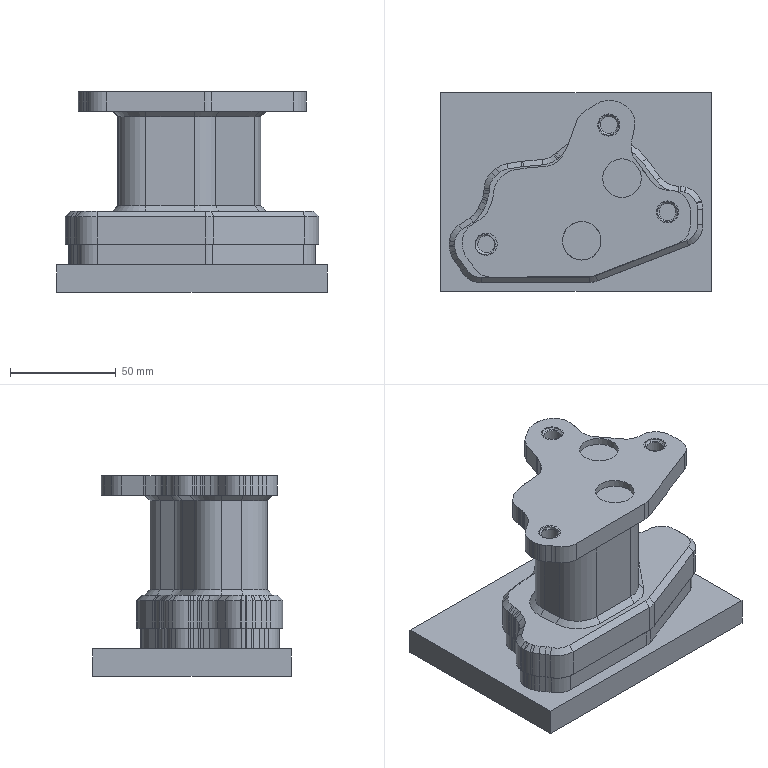NC program | NX | posted by the shop | part box 128.162 x 94.109 x 95 mm
Lines 31063 to 32055 of 131503:
31062 TOOL CALL 10 Z S8000
31063 CALL LBL101
31064 M3 M8
31065 M51
31066 CYCL DEF 32.0 TOLERANCE
31067 CYCL DEF 32.1 T0.012
31068 CYCL DEF 32.2 HSC-MODE:0
31069 L M126
31070 PLANE SPATIAL SPA-90. SPB+0.0 SPC-179.758 TURN FMAX SEQ-
31071 L X28.6141 Y32.9464 FMAX
31072 L Z140. FMAX
31073 L X28.614 Z35.4807 FMAX
31074 L X25.014 F1000.
31075 L Y14.5684
31076 L X24.4525 Y14.6761
31077 L X23.2391 Y14.816
31078 L X22.072 Y14.8611
31079 L X22.014
31080 L X-1.056
31081 L X-1.973 Y14.8323
31082 L X-2.9301 Y14.7461
31083 L X-3.8765 Y14.6024
31084 L X-4.0089 Y14.5747
31085 L Y51.3242
31086 L X-3.4472 Y51.2166
31087 L X-2.234 Y51.0768
31088 L X-1.0669 Y51.0316
31089 L X-1.0089
31090 L X22.0611
31091 L X22.9781 Y51.0604
31092 L X23.9352 Y51.1467
31093 L X24.8816 Y51.2903
31094 L X25.014 Y51.318
31095 L Y32.9464
31096 L X22.014
31097 L Y17.8611
31098 L X-1.0089
31099 L Y48.0316
31100 L X22.014
31101 L Y32.9464
31102 L X19.014
31103 L Y20.8611
31104 L X1.9911
31105 L Y45.0316
31106 L X19.014
31107 L Y32.9464
31108 L X16.014
31109 L Y23.8611
31110 L X4.9911
31111 L Y42.0316
31112 L X16.014
31113 L Y32.9464
31114 L X13.014
31115 L Y26.8611
31116 L X7.9911
31117 L Y39.0316
31118 L X10.4911
31119 L Y36.5316
31120 L X10.514
31121 L Y29.3611
31122 L X10.4911
31123 L Y36.5316
31124 L Y39.0316
31125 L X13.014
31126 L Y32.9464
31127 L X16.614
31128 L Z140. FMAX
31129 PLANE RESET STAY
31130 * - OPERATION: 新底壁铣_1_COPY - TOOL: T10 J-D6R0.5
31131 CALL LBL101
31132 CYCL DEF 32.0 TOLERANCE
31133 CYCL DEF 32.1 T0.012
31134 CYCL DEF 32.2 HSC-MODE:0
31135 PLANE SPATIAL SPA-90. SPB+0.0 SPC-3.662 TURN FMAX SEQ-
31136 L X1.7819 Y32.9464 FMAX
31137 L Z140. FMAX
31138 L X1.7818 Z20.4544 FMAX
31139 L X5.3818 F1000.
31140 L Y51.3246
31141 L X5.9427 Y51.2171
31142 L X7.1562 Y51.0765
31143 L X8.3242 Y51.0316
31144 L X8.3818
31145 L X14.9774
31146 L X15.8945 Y51.0604
31147 L X16.8516 Y51.1467
31148 L X17.798 Y51.2903
31149 L X17.9304 Y51.318
31150 L Y14.5685
31151 L X17.3687 Y14.6761
31152 L X16.1555 Y14.816
31153 L X14.9884 Y14.8611
31154 L X14.9304
31155 L X8.3347
31156 L X7.4177 Y14.8323
31157 L X6.4606 Y14.7461
31158 L X5.5141 Y14.6024
31159 L X5.3818 Y14.5747
31160 L Y32.9464
31161 L X8.3818
31162 L Y48.0316
31163 L X14.9304
31164 L Y17.8611
31165 L X8.3818
31166 L Y32.9464
31167 L X11.3818
31168 L Y45.0316
31169 L X11.9304
31170 L Y20.8611
31171 L X11.3818
31172 L Y32.9464
31173 L X7.7818
31174 L Z140. FMAX
31175 PLANE RESET STAY
31176 * - OPERATION: 等高混合 - TOOL: T10 J-D6R0.5
31177 CALL LBL101
31178 CYCL DEF 32.0 TOLERANCE
31179 CYCL DEF 32.1 T0.006
31180 CYCL DEF 32.2 HSC-MODE:0
31181 PLANE SPATIAL SPA-90. SPB+0.0 SPC+0.0 TURN FMAX SEQ-
31182 L X13.296 Y14.3074 FMAX
31183 L Z83.7547 FMAX
31184 L Z43.2547 FMAX
31185 CC X15.296 Y14.3211
31186 C X15.296 Y12.3211 DR+ F250.
31187 L X16.7642 F2500.
31188 L X16.8776 Y12.3206 Z43.247
31189 L X16.9909 Y12.3211 Z43.2393
31190 L X17.1042 Z43.2316
31191 L X17.2176 Z43.2239
31192 L X17.3309 Y12.3204 Z43.2162
31193 L X17.4442 Y12.3211 Z43.2085
31194 L X17.5576 Z43.2008
31195 L X17.6709 Z43.1932
31196 L X17.7842 Y12.3205 Z43.1855
31197 L X17.8976 Y12.3211 Z43.1778
31198 L X18.0109 Z43.1701
31199 L X18.1242 Z43.1624
31200 L X18.2375 Z43.1547
31201 L X13.5829
31202 L X13.5432 Y12.3207
31203 L X13.4221 Y12.3211 Z43.1347
31204 L X13.0586 Z43.0747
31205 L X12.9374 Y12.3206 Z43.0547
31206 L X13.0935 Y12.3211
31207 L X18.7348
31208 L X18.8509 Y12.3205
31209 L X18.9714 Y12.3211 Z43.0297
31210 L X19.0919 Z43.0047
31211 L X19.2123 Z42.9797
31212 L X19.3328 Y12.3205 Z42.9547
31213 L X12.4526 Y12.3204
31214 L X12.3573 Y12.3211 Z42.9297
31215 L X12.262 Z42.9047
31216 L X12.1667 Z42.8797
31217 L X12.0714 Z42.8547
31218 L X19.7213 Y12.3207
31219 L X19.8299 Y12.3204 Z42.8214
31220 L X19.9385 Y12.3211 Z42.788
31221 L X20.0471 Y12.3201 Z42.7547
31222 L X11.7317 Y12.3199
31223 L X11.6327 Y12.3211 Z42.7214
31224 L X11.5338 Z42.688
31225 L X11.4348 Y12.3203 Z42.6547
31226 L X20.3518 Y12.3201
31227 L X20.4405 Y12.321 Z42.6214
31228 L X20.5292 Z42.588
31229 L X20.6179 Y12.3202 Z42.5547
31230 L X20.4789 Y12.3211
31231 L X16.8018
31232 L X15.1344
31233 L X11.1511 Y12.321
31234 L X11.0302 Z42.5047
31235 L X10.9092 Z42.4547
31236 L X13.5853 Y12.3211
31237 L X18.2187
31238 L X20.7078
31239 L X20.859 Y12.3198
31240 L X20.941 Y12.3211 Z42.4214
31241 L X21.023 Z42.388
31242 L X21.1049 Z42.3547
31243 L X18.8143
31244 L X12.9705
31245 L X10.9568
31246 L X10.6732 Y12.3207
31247 L X10.5642 Y12.3209 Z42.3047
31248 L X10.4553 Y12.3201 Z42.2547
31249 L X10.6464 Y12.3211
31250 L X12.5219
31251 L X19.2578
31252 L X21.1691
31253 L X21.3186 Y12.3207
31254 L X21.4254 Y12.321 Z42.2047
31255 L X21.5322 Y12.3211 Z42.1547
31256 L X19.624
31257 L X12.1519
31258 L X10.4016
31259 L X10.2511 Y12.3194
31260 L X10.1521 Y12.321 Z42.1047
31261 L X10.0532 Y12.3193 Z42.0547
31262 L X10.1569 Y12.3211
31263 L X11.8326
31264 L X19.9416
31265 L X21.7212
31266 L X21.8126 Y12.3209 Z42.0047
31267 L X21.9041 Y12.3211 Z41.9547
31268 L X20.226
31269 L X11.5476
31270 L X9.9122
31271 L X9.864 Y12.3206
31272 L X9.7776 Y12.321 Z41.9047
31273 L X9.6912 Y12.3206 Z41.8547
31274 L X9.8348 Y12.3211
31275 L X11.2888
31276 L X20.4836
31277 L X22.0868 Y12.3209
31278 L X22.1732 Z41.8047
31279 L X22.2597 Z41.7547
31280 L X20.7218 Y12.3211
31281 L X11.0504
31282 L X9.6675
31283 L X9.5185 Y12.3193
31284 L X9.4347 Y12.321 Z41.7047
31285 L X9.351 Y12.3194 Z41.6547
31286 L X9.4228 Y12.3211
31287 L X10.8296
31288 L X20.9423
31289 L X22.413
31290 L X22.4297 Y12.3206
31291 L X22.5147 Y12.3209 Z41.6047
31292 L X22.5998 Y12.3207 Z41.5547
31293 L X22.5756 Y12.3211
31294 L X21.1501
31295 L X10.6218
31296 L X9.1898 Y12.3209
31297 L X9.1092 Y12.3204 Z41.5047
31298 L X9.0287 Y12.3192 Z41.4547
31299 L X9.1781 Y12.3211
31300 L X10.4257
31301 L X21.3451
31302 L X22.7571
31303 L X22.7724 Y12.3206
31304 L X22.8646 Y12.3204 Z41.4047
31305 L X22.9567 Y12.3196 Z41.3547
31306 L X22.8821 Y12.3211
31307 L X21.53
31308 L X10.2409
31309 L X8.9334
31310 L X8.8676 Y12.3195
31311 L X8.787 Y12.321 Z41.3047
31312 L X8.7064 Y12.3207 Z41.2547
31313 L X9.9122 Y12.3211
31314 L X10.0649
31315 L X21.7063
31316 L X23.0792 Y12.3209
31317 L X23.1794 Y12.3211 Z41.2047
31318 L X23.2797 Z41.1547
31319 L X21.8772
31320 L X9.8967
31321 L X8.6886
31322 L X8.5453 Y12.3192
31323 L X8.4647 Y12.321 Z41.1047
31324 L X8.3842 Y12.3196 Z41.0547
31325 L X8.4439 Y12.3211
31326 L X9.734
31327 L X22.0472
31328 L X23.4515 Y12.321
31329 L X23.5331 Y12.3209 Z41.0047
31330 L X23.6147 Y12.3207 Z40.9547
31331 L X22.2172 Y12.3211
31332 L X9.5728
31333 L X8.4439
31334 L X8.223 Y12.3206
31335 L X8.1425 Y12.3204 Z40.9047
31336 L X8.0619 Y12.3191 Z40.8547
31337 L X8.1992 Y12.3211
31338 L X9.4117
31339 L X22.3872
31340 L X23.7652
31341 L X23.8439 Y12.321 Z40.8047
31342 L X23.9227 Y12.3211 Z40.7547
31343 L X22.5572
31344 L X9.2506
31345 L X7.9008
31346 L X7.8202 Y12.3203 Z40.7047
31347 L X7.7397 Y12.3204 Z40.6547
31348 L X7.8982 Y12.3211
31349 L X9.0895
31350 L X22.7272
31351 L X24.0581
31352 L X24.1287 Y12.321 Z40.6047
31353 L X24.1994 Y12.3211 Z40.5547
31354 L X22.8972
31355 L X8.9283
31356 L X7.7098
31357 L X7.5786 Y12.3191
31358 L X7.498 Y12.321 Z40.5047
31359 L X7.4174 Y12.3198 Z40.4547
31360 L X7.4651 Y12.3211
31361 L X8.7672
31362 L X23.0659
31363 L X24.3368 Y12.321
31364 L X24.4048 Z40.4047
31365 L X24.4729 Y12.3211 Z40.3547
31366 L X23.2294
31367 L X8.6061
31368 L X7.4651
31369 L X7.2563 Y12.3202
31370 L X7.1686 Y12.3209 Z40.3047
31371 L X7.0809 Y12.3187 Z40.2547
31372 L X7.2203 Y12.3211
31373 L X8.445
31374 L X23.3859
31375 L X24.5946
31376 L X24.715 Y12.3208 Z40.1547
31377 L X23.5361 Y12.3211
31378 L X8.2838
31379 L X6.9756
31380 L X6.8533 Y12.3176
31381 L Y12.3205 Z40.0547
31382 L X6.9756 Y12.3211
31383 L X8.1227
31384 L X23.6804
31385 L X24.8363 Y12.321
31386 L X24.9575 Y12.3211 Z39.9547
31387 L X23.8193
31388 L X7.9616
31389 L X6.6118 Y12.3191
31390 L X6.5313 Y12.3209 Z39.9047
31391 L X6.4507 Y12.3206 Z39.8547
31392 L X6.4862 Y12.3211
31393 L X7.8005
31394 L X23.953
31395 L X25.0833 Y12.3204
31396 L X25.1705 Y12.3211 Z39.7547
31397 L X24.082
31398 L X7.6393
31399 L X6.4185
31400 L X6.2896 Y12.32
31401 L X6.209 Y12.321 Z39.7047
31402 L X6.1285 Y12.3191 Z39.6547
31403 L X6.2415 Y12.3211
31404 L X7.4782
31405 L X24.2066
31406 L X25.2803 Y12.321
31407 L X25.3978 Y12.3204 Z39.5547
31408 L X25.3751 Y12.3211
31409 L X24.327
31410 L X7.3171
31411 L X5.9674 Y12.3209
31412 L X5.8868 Y12.321 Z39.5047
31413 L X5.8062 Y12.3199 Z39.4547
31414 L X5.9516 Y12.3211
31415 L X7.156
31416 L X24.4436
31417 L X25.4771
31418 L X25.5006 Y12.3203
31419 L X25.5771 Y12.3211 Z39.3547
31420 L X24.5559
31421 L X6.9948
31422 L X5.752
31423 L X5.6451 Y12.3193
31424 L X5.5645 Y12.3209 Z39.3047
31425 L X5.4839 Y12.3204 Z39.2547
31426 L X5.5073 Y12.3211
31427 L X6.8337
31428 L X24.6647
31429 L X25.6708 Y12.3207
31430 L X25.7646 Y12.3206 Z39.1547
31431 L X24.7702 Y12.3211
31432 L X6.6726
31433 L X5.5073
31434 L X5.3228 Y12.3197
31435 L X5.2423 Y12.3204 Z39.1047
31436 L X5.1618 Y12.3203 Z39.0547
31437 L X5.1895 Y12.3211
31438 L X6.5115
31439 L X24.8727
31440 L X25.8577 Y12.3208
31441 L X25.9431 Y12.3207 Z38.9547
31442 L X24.9724 Y12.3211
31443 L X6.3503
31444 L X5.0179
31445 L X5.0006 Y12.3206
31446 L X4.92 Y12.3209 Z38.9047
31447 L X4.8395 Y12.3204 Z38.8547
31448 L X4.8718 Y12.3211
31449 L X6.1892
31450 L X25.0687
31451 L X26.0257 Y12.3208
31452 L X26.1082 Y12.3206 Z38.7547
31453 L X26.0727 Y12.3211
31454 L X25.1621
31455 L X6.0281
31456 L X4.7732
31457 L X4.6784 Y12.3194
31458 L X4.5978 Y12.3209 Z38.7047
31459 L X4.5172 Y12.3207 Z38.6547
31460 L X5.867 Y12.3211
31461 L X25.2533
31462 L X26.1907 Y12.3209
31463 L X26.3028 Y12.3203 Z38.5547
31464 L X26.238 Y12.3211
31465 L X25.3422
31466 L X5.7058
31467 L X4.3562 Y12.3197
31468 L X4.2756 Y12.321 Z38.5047
31469 L X4.195 Y12.3204 Z38.4547
31470 L X4.2838 Y12.3211
31471 L X5.5447
31472 L X25.4278
31473 L X26.3326 Y12.321
31474 L X26.4227 Y12.3211 Z38.3547
31475 L X25.5115
31476 L X5.3836
31477 L X4.039
31478 L X3.9789 Y12.3192
31479 L X3.8875 Y12.3209 Z38.2547
31480 L X5.2225 Y12.3211
31481 L X25.5935
31482 L X26.5131 Y12.3206
31483 L X26.5742 Y12.3207 Z38.1547
31484 L X25.6723 Y12.3211
31485 L X5.0613
31486 L X3.7943
31487 L X3.7165 Y12.3193
31488 L X3.6407 Y12.321 Z38.1047
31489 L X3.5649 Y12.3211 Z38.0547
31490 L X4.9002
31491 L X25.7504
31492 L X26.6466
31493 L X26.7192 Y12.3209 Z37.9547
31494 L X25.8277 Y12.3211
31495 L X4.7391
31496 L X3.5496
31497 L X3.4142 Y12.3195
31498 L X3.3407 Y12.3203 Z37.9047
31499 L X3.2673 Y12.3201 Z37.8547
31500 L X3.3049 Y12.3211
31501 L X4.578
31502 L X25.9039
31503 L X26.7914 Y12.3209
31504 L X26.8554 Y12.3205 Z37.7547
31505 L X25.9789 Y12.3211
31506 L X4.4168
31507 L X3.1306 Y12.321
31508 L X3.0644 Y12.3209 Z37.7047
31509 L X2.9983 Y12.32 Z37.6547
31510 L X3.0602 Y12.3211
31511 L X4.2557
31512 L X26.0518
31513 L X26.9192 Y12.3206
31514 L X26.9829 Z37.5547
31515 L X26.1225 Y12.3211
31516 L X4.0962
31517 L X2.9276
31518 L X2.866 Y12.3202
31519 L X2.8014 Y12.3209 Z37.5047
31520 L X2.7368 Y12.3211 Z37.4547
31521 L X3.9417
31522 L X26.1916
31523 L X27.0471 Y12.321
31524 L X27.1108 Y12.3208 Z37.3547
31525 L X26.259 Y12.3211
31526 L X3.7934
31527 L X2.7366
31528 L X2.6199 Y12.3199
31529 L X2.5034 Y12.3203 Z37.2547
31530 L X2.5457 Y12.3211
31531 L X3.6509
31532 L X26.324
31533 L X27.123 Y12.321
31534 L X27.1693 Y12.3207
31535 L X27.2248 Y12.3206 Z37.1547
31536 L X27.1775 Y12.321
31537 L X26.3879 Y12.3211
31538 L X3.5137
31539 L X2.4117
31540 L X2.3867 Y12.3207
31541 L X2.2745 Y12.3199 Z37.0547
31542 L X2.326 Y12.3211
31543 L X3.3815
31544 L X26.4497
31545 L X27.2804 Y12.3208
31546 L X27.336 Y12.3204 Z36.9547
31547 L X27.3063 Y12.321
31548 L X26.4725 Y12.3211
31549 L X3.2538
31550 L X2.1684 Y12.3205
31551 L X2.065 Y12.3207 Z36.8547
31552 L X2.0813 Y12.3211
31553 L X3.1307
31554 L X26.4725
31555 L X27.3658 Y12.321
31556 L X27.3916 Y12.3204
31557 L X27.4436 Y12.3205 Z36.7547
31558 L X27.4257 Y12.321
31559 L X26.4725 Y12.3211
31560 L X3.0116
31561 L X2.0199
31562 L X1.9621 Y12.3205
31563 L X1.8439 Y12.3207 Z36.6547
31564 L X1.8597 Y12.3211
31565 L X2.8965
31566 L X26.4725
31567 L X27.4817 Y12.321
31568 L X27.5256 Y12.3205
31569 L X27.5781 Y12.3197 Z36.5547
31570 L X27.5451 Y12.3206
31571 L X26.4725 Y12.3211
31572 L X2.785
31573 L X1.8366
31574 L X1.7648 Y12.3197
31575 L X1.6735 Y12.3205 Z36.4547
31576 L X1.6922 Y12.3211
31577 L X2.6772
31578 L X26.4725
31579 L X27.605 Y12.3206
31580 L X27.626 Y12.3197
31581 L X27.6739 Y12.3202 Z36.3547
31582 L X26.4725 Y12.3211
31583 L X2.5724
31584 L X1.582 Y12.3208
31585 L X1.4919 Y12.3198 Z36.2547
31586 L X1.5388 Y12.3211
31587 L X2.4707
31588 L X26.4725
31589 L X27.4817 Y12.321
31590 L X27.7214 Y12.3205
31591 L X27.7594 Y12.3197 Z36.1547
31592 L X27.7196 Y12.3206
31593 L X26.4725 Y12.3211
31594 L X2.3718
31595 L X1.5388
31596 L X1.4024 Y12.3206
31597 L X1.3203 Y12.3203 Z36.0547
31598 L X1.3472 Y12.3211
31599 L X2.2765
31600 L X26.4725
31601 L X27.7779
31602 L X27.8012 Y12.32
31603 L X27.8451 Y12.3201 Z35.9547
31604 L X26.4725 Y12.3211
31605 L X2.1837
31606 L X1.2399 Y12.3209
31607 L X1.1591 Y12.3198 Z35.8547
31608 L X1.2353 Y12.3211
31609 L X2.0933
31610 L X26.4725
31611 L X27.8371 Y12.3206
31612 L X27.8858 Y12.3199
31613 L X27.9265 Y12.3197 Z35.7547
31614 L X27.9016 Y12.3206
31615 L X26.4725 Y12.3211
31616 L X2.0051
31617 L X1.0936
31618 L X1.0796 Y12.3206
31619 L X1.0039 Y12.3197 Z35.6547
31620 L X1.1025 Y12.3211
31621 L X1.9198
31622 L X26.4725
31623 L X27.9664 Y12.3203
31624 L X28.0002 Y12.3199 Z35.5547
31625 L X27.9616 Y12.3206
31626 L X26.4725 Y12.3211
31627 L X1.8369
31628 L X.9509
31629 L X.9295 Y12.3204
31630 L X.8583 Y12.3211 Z35.4547
31631 L X1.7558
31632 L X26.4725
31633 L X28.0212 Y12.3206
31634 L X28.0342 Y12.3199
31635 L X28.0702 Y12.3204 Z35.3547
31636 L X26.4725 Y12.3211
31637 L X1.6767
31638 L X.8135
31639 L X.7877 Y12.3203
31640 L X.7167 Y12.3201 Z35.2547
31641 L X.8135 Y12.3211
31642 L X1.6003
31643 L X26.4725
31644 L X28.0727 Y12.3206
31645 L X28.1017 Y12.3198
31646 L X28.1355 Y12.3205 Z35.1547
31647 L X26.4725 Y12.3211
31648 L X1.5258
31649 L X.6775
31650 L X.6484 Y12.3204
31651 L X.5848 Z35.0547
31652 L X.613 Y12.3211
31653 L X1.4531
31654 L X26.4725
31655 L X28.1361 Y12.3206
31656 L X28.1654 Y12.3196
31657 L X28.1947 Y12.3205 Z34.9547
31658 L X26.4725 Y12.3211
31659 L X1.3821
31660 L X.5458
31661 L X.5229 Y12.3203
31662 L X.4607 Y12.32 Z34.8547
31663 L X.5458 Y12.3211
31664 L X1.3136
31665 L X26.4725
31666 L X28.195 Y12.3206
31667 L X28.2219 Y12.3196
31668 L X28.2492 Y12.3206 Z34.7547
31669 L X26.4725 Y12.3211
31670 L X1.2467
31671 L X.4149
31672 L X.3985 Y12.3207
31673 L X.3376 Y12.3203 Z34.6547
31674 L X.3683 Y12.3211
31675 L X1.1813
31676 L X26.4725
31677 L X28.2659 Y12.3206
31678 L X28.2833 Y12.3199
31679 L X28.3033 Y12.3204 Z34.5547
31680 L X26.4725 Y12.3211
31681 L X1.118
31682 L X.2795 Y12.3206
31683 L X.2256 Y12.321 Z34.4547
31684 L X1.0566 Y12.3211
31685 L X26.4725
31686 L X28.3058 Y12.3206
31687 L X28.3318 Y12.3196
31688 L X28.3319 Y12.3202 Z34.3547
31689 L X26.4725 Y12.3211
31690 L X.9967
31691 L X.1717 Y12.3209
31692 L X.1177 Y12.321 Z34.2547
31693 L X.9382 Y12.3211
31694 L X26.4725
31695 L X28.363 Y12.3206
31696 L X28.3917 Y12.3191
31697 L X28.3918 Y12.3197 Z34.1547
31698 L X28.363 Y12.3206
31699 L X26.4725 Y12.3211
31700 L X.8817
31701 L X.0638 Y12.321
31702 L X.0126 Y12.3209 Z34.0547
31703 L X.8268 Y12.3211
31704 L X26.4725
31705 L X28.3918 Y12.3203
31706 L X28.452 Y12.3191 Z33.9547
31707 L X28.4257 Y12.3206
31708 L X26.4725 Y12.3211
31709 L X.7734
31710 L X-.0336 Y12.321
31711 L X-.0799 Y12.3209 Z33.8547
31712 L X.7213 Y12.3211
31713 L X26.4725
31714 L X28.4257 Y12.3206
31715 L X28.4521 Y12.3196
31716 L Y12.3201 Z33.7547
31717 L X26.4725 Y12.3211
31718 L X.6712
31719 L X-.1262 Y12.3209
31720 L X-.1724 Y12.321 Z33.6547
31721 L X.622 Y12.3211
31722 L X26.4725
31723 L X28.4812 Y12.3204
31724 L X28.4972 Y12.32 Z33.5547
31725 L X28.4837 Y12.3206
31726 L X26.4725 Y12.3211
31727 L X.5746
31728 L X-.2187 Y12.321
31729 L X-.2601 Y12.3209 Z33.4547
31730 L X.5287 Y12.3211
31731 L X26.4725
31732 L X28.4972 Y12.3206
31733 L X28.5107 Z33.3547
31734 L X26.4725 Y12.3211
31735 L X.4837
31736 L X-.2991 Y12.3209
31737 L X-.3376 Z33.2547
31738 L X.4407 Y12.3211
31739 L X26.4725
31740 L X28.5109 Y12.3207
31741 L X28.511 Z33.1547
31742 L X26.4725 Y12.3211
31743 L X.3987
31744 L X-.3772 Y12.321
31745 L X-.4162 Y12.3209 Z33.0547
31746 L X.358 Y12.3211
31747 L X26.4725
31748 L X28.5112 Y12.3207
31749 L X28.5113 Z32.9547
31750 L X26.4725 Y12.3211
31751 L X.3189
31752 L X-.4552 Y12.3209
31753 L X-.491 Z32.8547
31754 L X.2806 Y12.3211
31755 L X26.4725
31756 L X28.5115 Y12.3208
31757 L X28.5116 Z32.7547
31758 L X26.4725 Y12.3211
31759 L X.244
31760 L X-.5265 Y12.3209
31761 L X-.562 Y12.3208 Z32.6547
31762 L X.2079 Y12.3211
31763 L X26.4725
31764 L X28.5117 Y12.3208
31765 L X28.5119 Y12.3209 Z32.5547
31766 L X26.4725 Y12.3211
31767 L X.1724
31768 L X-.5976 Y12.3208
31769 L X-.6331 Z32.4547
31770 L X.1368 Y12.3211
31771 L X26.4725
31772 L X28.512 Y12.3209
31773 L X28.5122 Z32.3547
31774 L X26.4725 Y12.3211
31775 L X.1013
31776 L X-.6686 Y12.3209
31777 L X-.7042 Z32.2547
31778 L X.0658 Y12.3211
31779 L X26.4725
31780 L X28.5123 Y12.321
31781 L X28.5125 Z32.1547
31782 L X26.4725 Y12.3211
31783 L X.0302
31784 L X-.7397 Y12.3208
31785 L X-.7753 Z32.0547
31786 L X-.0053 Y12.3211
31787 L X26.4725
31788 L X28.5126 Y12.321
31789 L X28.5128 Y12.3211 Z31.9547
31790 L X26.4725
31791 L X-.0409
31792 L X-.8108 Y12.321
31793 L X-.8463 Y12.3209 Z31.8547
31794 L X-.0764 Y12.3211
31795 L X26.4725
31796 L X28.5129
31797 L X28.513 Z31.7547
31798 L X26.4725
31799 L X-.1119
31800 L X-.8819 Y12.3207
31801 L X-.9174 Y12.321 Z31.6547
31802 L X-.1475 Y12.3211
31803 L X26.4725
31804 L X28.5132
31805 CC X28.5359 Y9.3206
31806 C X30.476 Y11.6097 DR-
31807 L Z31.5547
31808 L X30.4657 Y11.6181
31809 CC X28.5358 Y9.3212
31810 C X28.5133 Y12.3212 DR+
31811 L X26.4725 Y12.3211
31812 L X-.183
31813 L X-.9529 Y12.3209
31814 L X-.9885 Y12.3207 Z31.4547
31815 L X-.2185 Y12.3211
31816 L X26.4725
31817 L X28.5135 Y12.3212
31818 CC X28.5361 Y9.3224
31819 C X30.4643 Y11.6192 DR-
31820 L X30.476 Y11.6097
31821 L Z31.3547
31822 L X30.4629 Y11.6203
31823 CC X28.5362 Y9.3231
31824 C X28.5136 Y12.3212 DR+
31825 L X26.4725 Y12.3211
31826 L X-.2541
31827 L X-1.024 Y12.3208
31828 L X-1.0596 Z31.2548
31829 L X-.2896 Y12.3211
31830 L X26.4725
31831 L X28.5138 Y12.3212
31832 CC X28.5363 Y9.3239
31833 C X30.4614 Y11.6214 DR-
31834 L X30.476 Y11.6097
31835 L Z31.1548
31836 L X30.46 Y11.6225
31837 CC X28.5365 Y9.3247
31838 C X28.5139 Y12.3212 DR+
31839 L X26.4725 Y12.3211
31840 L X-.3252
31841 L X-1.0951 Y12.3208
31842 L X-1.1306 Y12.3207 Z31.0548
31843 L X-.3607 Y12.3211
31844 L X26.4725
31845 L X28.5141 Y12.3212
31846 CC X28.5367 Y9.3255
31847 C X30.4586 Y11.6236 DR-
31848 L X30.476 Y11.6097
31849 L Z30.9548
31850 L X30.4571 Y11.6247
31851 CC X28.5368 Y9.3263
31852 C X28.5142 Y12.3212 DR+
31853 L X26.4725 Y12.3211
31854 L X-.3962
31855 L X-1.1398 Y12.321
31856 L X-1.1662 Y12.3207
31857 L X-1.2017 Y12.3206 Z30.8548
31858 L X-1.1774 Y12.321
31859 L X-.4318 Y12.3211
31860 L X26.4725
31861 L X28.5144 Y12.3212
31862 CC X28.537 Y9.3271
31863 C X30.4557 Y11.6258 DR-
31864 L X30.476 Y11.6097
31865 L Z30.7548
31866 L X30.4543 Y11.6268
31867 CC X28.5372 Y9.3281
31868 C X28.5145 Y12.3212 DR+
31869 L X26.4725 Y12.3211
31870 L X-.4673
31871 L X-1.2159 Y12.321
31872 L X-1.2372 Y12.3206
31873 L X-1.2727 Z30.6549
31874 L X-1.2553 Y12.321
31875 L X-.5028 Y12.3211
31876 L X26.4725
31877 L X28.5146 Y12.3212
31878 CC X28.5374 Y9.329
31879 C X30.4528 Y11.6279 DR-
31880 L X30.476 Y11.6097
31881 L Z30.5549
31882 L X30.4514 Y11.629
31883 CC X28.5376 Y9.3298
31884 C X28.5148 Y12.3212 DR+
31885 L X26.4725 Y12.3211
31886 L X-.5383
31887 L X-1.3083 Y12.3206
31888 L X-1.3438 Y12.321 Z30.455
31889 L X-.5739 Y12.3211
31890 L X26.4725
31891 L X28.5149 Y12.3212
31892 CC X28.5378 Y9.3307
31893 C X30.45 Y11.6301 DR-
31894 L X30.476 Y11.6097
31895 L Z30.355
31896 L X30.4485 Y11.6312
31897 CC X28.538 Y9.3315
31898 C X28.5151 Y12.3212 DR+
31899 L X26.4725 Y12.3211
31900 L X-.6094
31901 L X-1.3793 Y12.3209
31902 L X-1.4148 Y12.321 Z30.2551
31903 L X-.6449 Y12.3211
31904 L X26.4725
31905 L X28.5152 Y12.3212
31906 CC X28.5381 Y9.3323
31907 C X30.4471 Y11.6323 DR-
31908 L X30.476 Y11.6097
31909 L Z30.1552
31910 L X30.4456 Y11.6334
31911 CC X28.5383 Y9.3331
31912 C X28.5154 Y12.3212 DR+
31913 L X26.4725 Y12.3211
31914 L X-.6804
31915 L X-1.4503 Y12.3208
31916 L X-1.4858 Y12.3206 Z30.0552
31917 L X-1.4613 Y12.321
31918 L X-.7159 Y12.3211
31919 L X26.4725
31920 L X28.5155 Y12.3212
31921 CC X28.5385 Y9.3339
31922 C X30.4442 Y11.6345 DR-
31923 L X30.476 Y11.6097
31924 L Z29.9553
31925 L X30.4428 Y11.6356
31926 CC X28.5386 Y9.3347
31927 C X28.5157 Y12.3212 DR+
31928 L X26.4725 Y12.3211
31929 L X-.7514
31930 L X-1.5047 Y12.321
31931 L X-1.5213 Y12.3206
31932 L X-1.5568 Y12.3207 Z29.8554
31933 L X-.7869 Y12.3211
31934 L X26.4725
31935 L X28.5158 Y12.3212
31936 CC X28.5388 Y9.3355
31937 C X30.4413 Y11.6367 DR-
31938 L X30.476 Y11.6097
31939 L Z29.7556
31940 L X30.4399 Y11.6378
31941 CC X28.539 Y9.3363
31942 C X28.516 Y12.3212 DR+
31943 L X26.4725 Y12.3211
31944 L X-.8224
31945 L X-1.5923 Y12.3209
31946 L X-1.6278 Y12.3207 Z29.6557
31947 L X-.8579 Y12.3211
31948 L X26.4725
31949 L X28.5161 Y12.3212
31950 CC X28.5391 Y9.337
31951 C X30.4385 Y11.6388 DR-
31952 L X30.476 Y11.6097
31953 L Z29.5558
31954 L X30.437 Y11.6399
31955 CC X28.5393 Y9.3378
31956 C X28.5162 Y12.3212 DR+
31957 L X26.4725 Y12.3211
31958 L X-.8934
31959 L X-1.6633 Y12.3209
31960 L X-1.6988 Y12.3206 Z29.456
31961 L X-1.6838 Y12.321
31962 L X-.9289 Y12.3211
31963 L X26.4725
31964 L X28.5164 Y12.3212
31965 CC X28.5394 Y9.3385
31966 C X30.4356 Y11.641 DR-
31967 L X30.476 Y11.6097
31968 L Z29.3561
31969 L X30.4342 Y11.6421
31970 CC X28.5396 Y9.3393
31971 C X28.5165 Y12.3212 DR+
31972 L X26.4725 Y12.3211
31973 L X-.9643
31974 L X-1.7343 Y12.3208
31975 L X-1.7698 Y12.3209 Z29.2563
31976 L X-.9998 Y12.3211
31977 L X26.4725
31978 L X28.5167 Y12.3212
31979 CC X28.5398 Y9.34
31980 C X30.4327 Y11.6432 DR-
31981 L X30.476 Y11.6097
31982 L Z29.1565
31983 L X30.4313 Y11.6443
31984 CC X28.5399 Y9.3407
31985 C X28.5168 Y12.3212 DR+
31986 L X26.4725 Y12.3211
31987 L X-1.0353
31988 L X-1.7775 Y12.321
31989 L X-1.8052 Y12.3206
31990 L X-1.8407 Y12.3208 Z29.0567
31991 L X-1.0708 Y12.3211
31992 L X26.4725
31993 L X28.517 Y12.3212
31994 CC X28.5401 Y9.3414
31995 C X30.4299 Y11.6454 DR-
31996 L X30.476 Y11.6097
31997 L Z28.957
31998 L X30.4285 Y11.6465
31999 CC X28.5402 Y9.3421
32000 C X28.5171 Y12.3212 DR+
32001 L X26.4725 Y12.3211
32002 L X-1.1062
32003 L X-1.8761 Y12.3208
32004 L X-1.9116 Y12.3207 Z28.8572
32005 L X-1.1417 Y12.3211
32006 L X26.4725
32007 L X28.5173 Y12.3212
32008 CC X28.5404 Y9.3428
32009 C X30.427 Y11.6476 DR-
32010 L X30.476 Y11.6097
32011 L Z28.7575
32012 L X30.4256 Y11.6487
32013 CC X28.5405 Y9.3435
32014 C X28.5174 Y12.3212 DR+
32015 L X26.4725 Y12.3211
32016 L X-1.1771
32017 L X-1.92 Y12.321
32018 L X-1.947 Y12.3205
32019 L X-1.9825 Y12.3206 Z28.6578
32020 L X-1.2125 Y12.3211
32021 L X26.4725
32022 L X28.5175 Y12.3212
32023 CC X28.5407 Y9.3442
32024 C X30.4242 Y11.6497 DR-
32025 L X30.476 Y11.6097
32026 L Z28.5581
32027 L X30.4227 Y11.6508
32028 CC X28.5408 Y9.3449
32029 C X28.5177 Y12.3212 DR+
32030 L X26.4725 Y12.3211
32031 L X-1.248
32032 L X-2.0179 Y12.3209
32033 L X-2.0533 Y12.3206 Z28.4584
32034 L X-2.0194 Y12.321
32035 L X-1.2834 Y12.3211
32036 L X26.4725
32037 L X28.5178 Y12.3212
32038 CC X28.5409 Y9.3455
32039 C X30.4213 Y11.6519 DR-
32040 L X30.476 Y11.6097
32041 L Z28.3588
32042 L X30.4199 Y11.653
32043 CC X28.5411 Y9.3462
32044 C X28.518 Y12.3212 DR+
32045 L X26.4725 Y12.3211
32046 L X-1.3188
32047 L X-2.0887 Y12.3207
32048 L X-2.1241 Y12.3208 Z28.2591
32049 L X-1.3542 Y12.3211
32050 L X26.4725
32051 L X28.5181 Y12.3212
32052 CC X28.5413 Y9.3471
32053 C X30.4184 Y11.6541 DR-
32054 L X30.476 Y11.6097